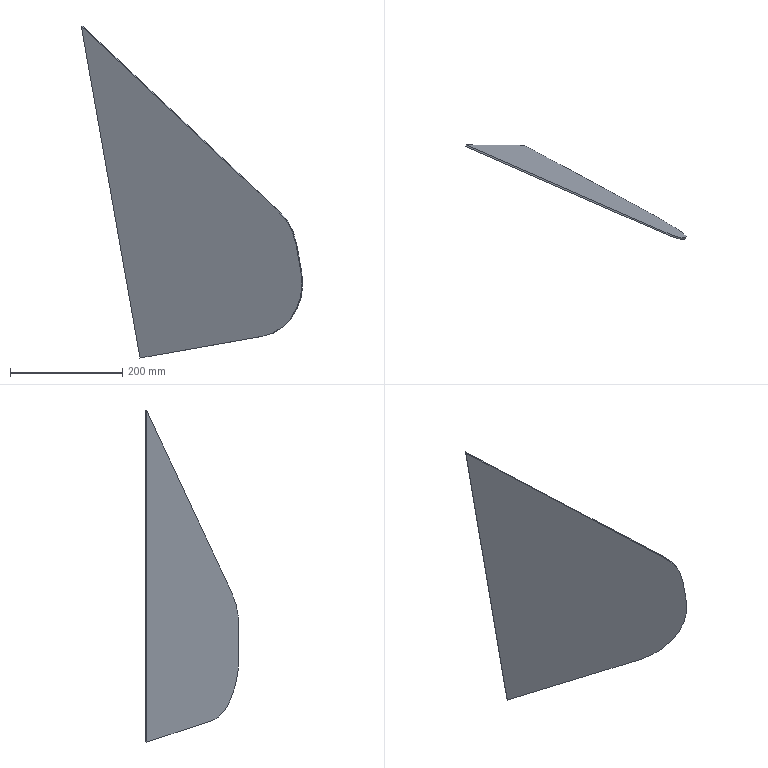Part | STEP file | floating channel right front section | 1 solid | 8 faces | box 394.503 x 166.964 x 591.584 mm | volume 406716 mm3 | plane 6 | cylinder 2 | commonest cylinder face diameters 200 x2
STEP:
#1=CARTESIAN_POINT('',(0.,0.,0.));
#2=DIRECTION('',(0.,0.,1.));
#3=DIRECTION('',(1.,0.,0.));
#4=AXIS2_PLACEMENT_3D('',#1,#2,#3);
#5=CARTESIAN_POINT('',(2381.907,-130.464,-318.268));
#6=VERTEX_POINT('',#5);
#7=CARTESIAN_POINT('',(2350.057,-119.338,-258.257));
#8=VERTEX_POINT('',#7);
#9=CARTESIAN_POINT('',(2294.958,-83.517,-333.629));
#10=DIRECTION('',(-0.4623,-0.8829,-0.08168));
#11=DIRECTION('',(0.8859,-0.4639,0.));
#12=AXIS2_PLACEMENT_3D('',#9,#10,#11);
#13=CIRCLE('',#12,100.);
#14=CARTESIAN_POINT('',(2294.958,-83.517,-333.629));
#15=DIRECTION('',(0.4623,0.8829,0.08168));
#16=DIRECTION('',(0.8859,-0.4639,0.));
#17=AXIS2_PLACEMENT_3D('',#14,#15,#16);
#18=CYLINDRICAL_SURFACE('',#17,100.);
#19=CARTESIAN_POINT('',(6.283,0.));
#20=DIRECTION('',(-1.,0.));
#21=VECTOR('',#20,1.);
#22=LINE('',#19,#21);
#23=(GEOMETRIC_REPRESENTATION_CONTEXT(2)PARAMETRIC_REPRESENTATION_CONTEXT()REPRESENTATION_CONTEXT('',''));
#24=DEFINITIONAL_REPRESENTATION('',(#22),#23);
#25=PCURVE('',#18,#24);
#26=CARTESIAN_POINT('',(443.818,847.627,78.409));
#27=DIRECTION('',(-0.4623,-0.8829,-0.08168));
#28=DIRECTION('',(-0.8859,0.4639,0.));
#29=AXIS2_PLACEMENT_3D('',#26,#27,#28);
#30=PLANE('',#29);
#31=CARTESIAN_POINT('',(-2071.861,413.419));
#32=DIRECTION('',(-1.,0.));
#33=AXIS2_PLACEMENT_2D('',#31,#32);
#34=CIRCLE('',#33,100.);
#35=(GEOMETRIC_REPRESENTATION_CONTEXT(2)PARAMETRIC_REPRESENTATION_CONTEXT()REPRESENTATION_CONTEXT('',''));
#36=DEFINITIONAL_REPRESENTATION('',(#34),#35);
#37=PCURVE('',#30,#36);
#38=SURFACE_CURVE('',#13,(#25,#37),.PCURVE_S1.);
#39=EDGE_CURVE('',#6,#8,#38,.T.);
#40=ORIENTED_EDGE('',*,*,#39,.F.);
#41=CARTESIAN_POINT('',(2383.294,-127.815,-318.023));
#42=VERTEX_POINT('',#41);
#43=CARTESIAN_POINT('',(2381.907,-130.464,-318.268));
#44=DIRECTION('',(-0.4623,-0.8829,-0.08168));
#45=VECTOR('',#44,1.);
#46=LINE('',#43,#45);
#47=CARTESIAN_POINT('',(6.128,0.));
#48=DIRECTION('',(0.,-1.));
#49=VECTOR('',#48,1.);
#50=LINE('',#47,#49);
#51=(GEOMETRIC_REPRESENTATION_CONTEXT(2)PARAMETRIC_REPRESENTATION_CONTEXT()REPRESENTATION_CONTEXT('',''));
#52=DEFINITIONAL_REPRESENTATION('',(#50),#51);
#53=PCURVE('',#18,#52);
#54=CARTESIAN_POINT('',(2408.119,-130.464,-466.64));
#55=DIRECTION('',(-0.8695,0.4695,-0.1536));
#56=DIRECTION('',(0.4751,0.8799,0.));
#57=AXIS2_PLACEMENT_3D('',#54,#55,#56);
#58=PLANE('',#57);
#59=CARTESIAN_POINT('',(-12.454,-150.154));
#60=DIRECTION('',(-0.9966,0.08266));
#61=VECTOR('',#60,1.);
#62=LINE('',#59,#61);
#63=(GEOMETRIC_REPRESENTATION_CONTEXT(2)PARAMETRIC_REPRESENTATION_CONTEXT()REPRESENTATION_CONTEXT('',''));
#64=DEFINITIONAL_REPRESENTATION('',(#62),#63);
#65=PCURVE('',#58,#64);
#66=SURFACE_CURVE('',#46,(#53,#65),.PCURVE_S1.);
#67=EDGE_CURVE('',#42,#6,#66,.T.);
#68=ORIENTED_EDGE('',*,*,#67,.F.);
#69=CARTESIAN_POINT('',(2351.444,-116.69,-258.012));
#70=VERTEX_POINT('',#69);
#71=CARTESIAN_POINT('',(2296.345,-80.868,-333.384));
#72=DIRECTION('',(0.4623,0.8829,0.08168));
#73=DIRECTION('',(0.8859,-0.4639,0.));
#74=AXIS2_PLACEMENT_3D('',#71,#72,#73);
#75=CIRCLE('',#74,100.);
#76=CARTESIAN_POINT('',(0.,3.));
#77=DIRECTION('',(1.,0.));
#78=VECTOR('',#77,1.);
#79=LINE('',#76,#78);
#80=(GEOMETRIC_REPRESENTATION_CONTEXT(2)PARAMETRIC_REPRESENTATION_CONTEXT()REPRESENTATION_CONTEXT('',''));
#81=DEFINITIONAL_REPRESENTATION('',(#79),#80);
#82=PCURVE('',#18,#81);
#83=CARTESIAN_POINT('',(445.205,850.276,78.654));
#84=DIRECTION('',(-0.4623,-0.8829,-0.08168));
#85=DIRECTION('',(-0.8859,0.4639,0.));
#86=AXIS2_PLACEMENT_3D('',#83,#84,#85);
#87=PLANE('',#86);
#88=CARTESIAN_POINT('',(-2171.861,413.419));
#89=CARTESIAN_POINT('',(-2171.861,586.624));
#90=CARTESIAN_POINT('',(-2021.861,500.022));
#91=CARTESIAN_POINT('',(-1871.861,413.419));
#92=CARTESIAN_POINT('',(-2021.861,326.816));
#93=CARTESIAN_POINT('',(-2171.861,240.214));
#94=CARTESIAN_POINT('',(-2171.861,413.419));
#95=(BOUNDED_CURVE()B_SPLINE_CURVE(2,(#88,#89,#90,#91,#92,#93,#94),.UNSPECIFIED.,.T.,.F.)B_SPLINE_CURVE_WITH_KNOTS((1,2,2,2,2,1),(-2.094,0.,2.094,4.189,6.283,8.378),.UNSPECIFIED.)CURVE()GEOMETRIC_REPRESENTATION_ITEM()RATIONAL_B_SPLINE_CURVE((1.,0.5,1.,0.5,1.,0.5,1.))REPRESENTATION_ITEM(''));
#96=(GEOMETRIC_REPRESENTATION_CONTEXT(2)PARAMETRIC_REPRESENTATION_CONTEXT()REPRESENTATION_CONTEXT('',''));
#97=DEFINITIONAL_REPRESENTATION('',(#95),#96);
#98=PCURVE('',#87,#97);
#99=SURFACE_CURVE('',#75,(#82,#98),.PCURVE_S1.);
#100=EDGE_CURVE('',#70,#42,#99,.T.);
#101=ORIENTED_EDGE('',*,*,#100,.F.);
#102=CARTESIAN_POINT('',(2350.057,-119.338,-258.257));
#103=DIRECTION('',(0.4623,0.8829,0.08168));
#104=VECTOR('',#103,1.);
#105=LINE('',#102,#104);
#106=CARTESIAN_POINT('',(5.426,0.));
#107=DIRECTION('',(0.,1.));
#108=VECTOR('',#107,1.);
#109=LINE('',#106,#108);
#110=(GEOMETRIC_REPRESENTATION_CONTEXT(2)PARAMETRIC_REPRESENTATION_CONTEXT()REPRESENTATION_CONTEXT('',''));
#111=DEFINITIONAL_REPRESENTATION('',(#109),#110);
#112=PCURVE('',#18,#111);
#113=CARTESIAN_POINT('',(2375.528,-130.464,-282.164));
#114=DIRECTION('',(-0.551,0.3582,-0.7537));
#115=DIRECTION('',(0.8073,0.,-0.5901));
#116=AXIS2_PLACEMENT_3D('',#113,#114,#115);
#117=PLANE('',#116);
#118=CARTESIAN_POINT('',(-34.672,-11.916));
#119=DIRECTION('',(0.325,-0.9457));
#120=VECTOR('',#119,1.);
#121=LINE('',#118,#120);
#122=(GEOMETRIC_REPRESENTATION_CONTEXT(2)PARAMETRIC_REPRESENTATION_CONTEXT()REPRESENTATION_CONTEXT('',''));
#123=DEFINITIONAL_REPRESENTATION('',(#121),#122);
#124=PCURVE('',#117,#123);
#125=SURFACE_CURVE('',#105,(#112,#124),.PCURVE_S1.);
#126=EDGE_CURVE('',#8,#70,#125,.T.);
#127=ORIENTED_EDGE('',*,*,#126,.F.);
#128=EDGE_LOOP('',(#40,#68,#101,#127));
#129=FACE_BOUND('',#128,.T.);
#130=ADVANCED_FACE('',(#129),#18,.T.);
#131=CARTESIAN_POINT('',(2321.171,-83.517,-482.001));
#132=VERTEX_POINT('',#131);
#133=CARTESIAN_POINT('',(2390.722,-130.464,-368.165));
#134=VERTEX_POINT('',#133);
#135=CARTESIAN_POINT('',(2303.774,-83.517,-383.526));
#136=DIRECTION('',(-0.4623,-0.8829,-0.08168));
#137=DIRECTION('',(0.8859,-0.4639,0.));
#138=AXIS2_PLACEMENT_3D('',#135,#136,#137);
#139=CIRCLE('',#138,100.);
#140=CARTESIAN_POINT('',(2303.774,-83.517,-383.526));
#141=DIRECTION('',(0.4623,0.8829,0.08168));
#142=DIRECTION('',(0.8859,-0.4639,0.));
#143=AXIS2_PLACEMENT_3D('',#140,#141,#142);
#144=CYLINDRICAL_SURFACE('',#143,100.);
#145=CARTESIAN_POINT('',(6.283,0.));
#146=DIRECTION('',(-1.,0.));
#147=VECTOR('',#146,1.);
#148=LINE('',#145,#147);
#149=(GEOMETRIC_REPRESENTATION_CONTEXT(2)PARAMETRIC_REPRESENTATION_CONTEXT()REPRESENTATION_CONTEXT('',''));
#150=DEFINITIONAL_REPRESENTATION('',(#148),#149);
#151=PCURVE('',#144,#150);
#152=CARTESIAN_POINT('',(-2079.671,463.483));
#153=DIRECTION('',(-1.,0.));
#154=AXIS2_PLACEMENT_2D('',#152,#153);
#155=CIRCLE('',#154,100.);
#156=(GEOMETRIC_REPRESENTATION_CONTEXT(2)PARAMETRIC_REPRESENTATION_CONTEXT()REPRESENTATION_CONTEXT('',''));
#157=DEFINITIONAL_REPRESENTATION('',(#155),#156);
#158=PCURVE('',#30,#157);
#159=SURFACE_CURVE('',#139,(#151,#158),.PCURVE_S1.);
#160=EDGE_CURVE('',#132,#134,#159,.T.);
#161=ORIENTED_EDGE('',*,*,#160,.F.);
#162=CARTESIAN_POINT('',(2322.558,-80.868,-481.756));
#163=VERTEX_POINT('',#162);
#164=CARTESIAN_POINT('',(2321.171,-83.517,-482.001));
#165=DIRECTION('',(-0.4623,-0.8829,-0.08168));
#166=VECTOR('',#165,1.);
#167=LINE('',#164,#166);
#168=CARTESIAN_POINT('',(1.416,0.));
#169=DIRECTION('',(0.,-1.));
#170=VECTOR('',#169,1.);
#171=LINE('',#168,#170);
#172=(GEOMETRIC_REPRESENTATION_CONTEXT(2)PARAMETRIC_REPRESENTATION_CONTEXT()REPRESENTATION_CONTEXT('',''));
#173=DEFINITIONAL_REPRESENTATION('',(#171),#172);
#174=PCURVE('',#144,#173);
#175=CARTESIAN_POINT('',(2103.8,33.851,-520.404));
#176=DIRECTION('',(-0.174,0.,0.9848));
#177=DIRECTION('',(-0.9848,0.,-0.174));
#178=AXIS2_PLACEMENT_3D('',#175,#176,#177);
#179=PLANE('',#178);
#180=CARTESIAN_POINT('',(-220.737,117.368));
#181=DIRECTION('',(0.4695,0.8829));
#182=VECTOR('',#181,1.);
#183=LINE('',#180,#182);
#184=(GEOMETRIC_REPRESENTATION_CONTEXT(2)PARAMETRIC_REPRESENTATION_CONTEXT()REPRESENTATION_CONTEXT('',''));
#185=DEFINITIONAL_REPRESENTATION('',(#183),#184);
#186=PCURVE('',#179,#185);
#187=SURFACE_CURVE('',#167,(#174,#186),.PCURVE_S1.);
#188=EDGE_CURVE('',#163,#132,#187,.T.);
#189=ORIENTED_EDGE('',*,*,#188,.F.);
#190=CARTESIAN_POINT('',(2392.109,-127.815,-367.92));
#191=VERTEX_POINT('',#190);
#192=CARTESIAN_POINT('',(2305.161,-80.868,-383.281));
#193=DIRECTION('',(0.4623,0.8829,0.08168));
#194=DIRECTION('',(0.8859,-0.4639,0.));
#195=AXIS2_PLACEMENT_3D('',#192,#193,#194);
#196=CIRCLE('',#195,100.);
#197=CARTESIAN_POINT('',(-6.283,3.));
#198=DIRECTION('',(1.,0.));
#199=VECTOR('',#198,1.);
#200=LINE('',#197,#199);
#201=(GEOMETRIC_REPRESENTATION_CONTEXT(2)PARAMETRIC_REPRESENTATION_CONTEXT()REPRESENTATION_CONTEXT('',''));
#202=DEFINITIONAL_REPRESENTATION('',(#200),#201);
#203=PCURVE('',#144,#202);
#204=CARTESIAN_POINT('',(-2179.671,463.483));
#205=CARTESIAN_POINT('',(-2179.671,636.688));
#206=CARTESIAN_POINT('',(-2029.671,550.086));
#207=CARTESIAN_POINT('',(-1879.671,463.483));
#208=CARTESIAN_POINT('',(-2029.671,376.881));
#209=CARTESIAN_POINT('',(-2179.671,290.278));
#210=CARTESIAN_POINT('',(-2179.671,463.483));
#211=(BOUNDED_CURVE()B_SPLINE_CURVE(2,(#204,#205,#206,#207,#208,#209,#210),.UNSPECIFIED.,.T.,.F.)B_SPLINE_CURVE_WITH_KNOTS((1,2,2,2,2,1),(-2.094,0.,2.094,4.189,6.283,8.378),.UNSPECIFIED.)CURVE()GEOMETRIC_REPRESENTATION_ITEM()RATIONAL_B_SPLINE_CURVE((1.,0.5,1.,0.5,1.,0.5,1.))REPRESENTATION_ITEM(''));
#212=(GEOMETRIC_REPRESENTATION_CONTEXT(2)PARAMETRIC_REPRESENTATION_CONTEXT()REPRESENTATION_CONTEXT('',''));
#213=DEFINITIONAL_REPRESENTATION('',(#211),#212);
#214=PCURVE('',#87,#213);
#215=SURFACE_CURVE('',#196,(#203,#214),.PCURVE_S1.);
#216=EDGE_CURVE('',#191,#163,#215,.T.);
#217=ORIENTED_EDGE('',*,*,#216,.F.);
#218=CARTESIAN_POINT('',(2390.722,-130.464,-368.165));
#219=DIRECTION('',(0.4623,0.8829,0.08168));
#220=VECTOR('',#219,1.);
#221=LINE('',#218,#220);
#222=CARTESIAN_POINT('',(-0.1547,0.));
#223=DIRECTION('',(0.,1.));
#224=VECTOR('',#223,1.);
#225=LINE('',#222,#224);
#226=(GEOMETRIC_REPRESENTATION_CONTEXT(2)PARAMETRIC_REPRESENTATION_CONTEXT()REPRESENTATION_CONTEXT('',''));
#227=DEFINITIONAL_REPRESENTATION('',(#225),#226);
#228=PCURVE('',#144,#227);
#229=CARTESIAN_POINT('',(-8.266,-99.658));
#230=DIRECTION('',(0.9966,-0.08266));
#231=VECTOR('',#230,1.);
#232=LINE('',#229,#231);
#233=(GEOMETRIC_REPRESENTATION_CONTEXT(2)PARAMETRIC_REPRESENTATION_CONTEXT()REPRESENTATION_CONTEXT('',''));
#234=DEFINITIONAL_REPRESENTATION('',(#232),#233);
#235=PCURVE('',#58,#234);
#236=SURFACE_CURVE('',#221,(#228,#235),.PCURVE_S1.);
#237=EDGE_CURVE('',#134,#191,#236,.T.);
#238=ORIENTED_EDGE('',*,*,#237,.F.);
#239=EDGE_LOOP('',(#161,#189,#217,#238));
#240=FACE_BOUND('',#239,.T.);
#241=ADVANCED_FACE('',(#240),#144,.T.);
#242=CARTESIAN_POINT('',(2000.716,36.5,71.181));
#243=VERTEX_POINT('',#242);
#244=CARTESIAN_POINT('',(2376.915,-127.815,-281.919));
#245=DIRECTION('',(-0.6948,0.3035,0.6521));
#246=VECTOR('',#245,1.);
#247=LINE('',#244,#246);
#248=CARTESIAN_POINT('',(-2165.016,361.782));
#249=DIRECTION('',(0.7562,-0.6543));
#250=VECTOR('',#249,1.);
#251=LINE('',#248,#250);
#252=(GEOMETRIC_REPRESENTATION_CONTEXT(2)PARAMETRIC_REPRESENTATION_CONTEXT()REPRESENTATION_CONTEXT('',''));
#253=DEFINITIONAL_REPRESENTATION('',(#251),#252);
#254=PCURVE('',#87,#253);
#255=CARTESIAN_POINT('',(0.9751,-2.837));
#256=DIRECTION('',(-0.9457,-0.325));
#257=VECTOR('',#256,1.);
#258=LINE('',#255,#257);
#259=(GEOMETRIC_REPRESENTATION_CONTEXT(2)PARAMETRIC_REPRESENTATION_CONTEXT()REPRESENTATION_CONTEXT('',''));
#260=DEFINITIONAL_REPRESENTATION('',(#258),#259);
#261=PCURVE('',#117,#260);
#262=SURFACE_CURVE('',#247,(#254,#261),.PCURVE_S1.);
#263=EDGE_CURVE('',#70,#243,#262,.T.);
#264=ORIENTED_EDGE('',*,*,#263,.F.);
#265=ORIENTED_EDGE('',*,*,#100,.T.);
#266=CARTESIAN_POINT('',(2409.506,-127.815,-466.395));
#267=DIRECTION('',(-0.174,0.,0.9848));
#268=VECTOR('',#267,1.);
#269=LINE('',#266,#268);
#270=CARTESIAN_POINT('',(-2193.888,546.876));
#271=DIRECTION('',(0.1541,-0.9881));
#272=VECTOR('',#271,1.);
#273=LINE('',#270,#272);
#274=(GEOMETRIC_REPRESENTATION_CONTEXT(2)PARAMETRIC_REPRESENTATION_CONTEXT()REPRESENTATION_CONTEXT('',''));
#275=DEFINITIONAL_REPRESENTATION('',(#273),#274);
#276=PCURVE('',#87,#275);
#277=CARTESIAN_POINT('',(2.99,-0.248));
#278=DIRECTION('',(-0.08266,-0.9966));
#279=VECTOR('',#278,1.);
#280=LINE('',#277,#279);
#281=(GEOMETRIC_REPRESENTATION_CONTEXT(2)PARAMETRIC_REPRESENTATION_CONTEXT()REPRESENTATION_CONTEXT('',''));
#282=DEFINITIONAL_REPRESENTATION('',(#280),#281);
#283=PCURVE('',#58,#282);
#284=SURFACE_CURVE('',#269,(#276,#283),.PCURVE_S1.);
#285=EDGE_CURVE('',#191,#42,#284,.T.);
#286=ORIENTED_EDGE('',*,*,#285,.F.);
#287=ORIENTED_EDGE('',*,*,#216,.T.);
#288=CARTESIAN_POINT('',(2105.187,36.5,-520.159));
#289=VERTEX_POINT('',#288);
#290=CARTESIAN_POINT('',(2105.187,36.5,-520.159));
#291=DIRECTION('',(0.8695,-0.4695,0.1536));
#292=VECTOR('',#291,1.);
#293=LINE('',#290,#292);
#294=CARTESIAN_POINT('',(-1848.07,600.82));
#295=DIRECTION('',(-0.9881,-0.1541));
#296=VECTOR('',#295,1.);
#297=LINE('',#294,#296);
#298=(GEOMETRIC_REPRESENTATION_CONTEXT(2)PARAMETRIC_REPRESENTATION_CONTEXT()REPRESENTATION_CONTEXT('',''));
#299=DEFINITIONAL_REPRESENTATION('',(#297),#298);
#300=PCURVE('',#87,#299);
#301=CARTESIAN_POINT('',(-1.408,-2.649));
#302=DIRECTION('',(-0.8829,0.4695));
#303=VECTOR('',#302,1.);
#304=LINE('',#301,#303);
#305=(GEOMETRIC_REPRESENTATION_CONTEXT(2)PARAMETRIC_REPRESENTATION_CONTEXT()REPRESENTATION_CONTEXT('',''));
#306=DEFINITIONAL_REPRESENTATION('',(#304),#305);
#307=PCURVE('',#179,#306);
#308=SURFACE_CURVE('',#293,(#300,#307),.PCURVE_S1.);
#309=EDGE_CURVE('',#289,#163,#308,.T.);
#310=ORIENTED_EDGE('',*,*,#309,.F.);
#311=CARTESIAN_POINT('',(2000.716,36.5,71.181));
#312=DIRECTION('',(0.174,0.,-0.9848));
#313=VECTOR('',#312,1.);
#314=LINE('',#311,#313);
#315=CARTESIAN_POINT('',(-1755.518,7.498));
#316=DIRECTION('',(-0.1541,0.9881));
#317=VECTOR('',#316,1.);
#318=LINE('',#315,#317);
#319=(GEOMETRIC_REPRESENTATION_CONTEXT(2)PARAMETRIC_REPRESENTATION_CONTEXT()REPRESENTATION_CONTEXT('',''));
#320=DEFINITIONAL_REPRESENTATION('',(#318),#319);
#321=PCURVE('',#87,#320);
#322=CARTESIAN_POINT('',(1999.329,33.851,70.936));
#323=DIRECTION('',(0.8695,-0.4695,0.1536));
#324=DIRECTION('',(-0.4751,-0.8799,0.));
#325=AXIS2_PLACEMENT_3D('',#322,#323,#324);
#326=PLANE('',#325);
#327=CARTESIAN_POINT('',(-2.99,-0.248));
#328=DIRECTION('',(-0.08266,0.9966));
#329=VECTOR('',#328,1.);
#330=LINE('',#327,#329);
#331=(GEOMETRIC_REPRESENTATION_CONTEXT(2)PARAMETRIC_REPRESENTATION_CONTEXT()REPRESENTATION_CONTEXT('',''));
#332=DEFINITIONAL_REPRESENTATION('',(#330),#331);
#333=PCURVE('',#326,#332);
#334=SURFACE_CURVE('',#314,(#321,#333),.PCURVE_S1.);
#335=EDGE_CURVE('',#243,#289,#334,.T.);
#336=ORIENTED_EDGE('',*,*,#335,.F.);
#337=EDGE_LOOP('',(#264,#265,#286,#287,#310,#336));
#338=FACE_BOUND('',#337,.T.);
#339=ADVANCED_FACE('',(#338),#87,.F.);
#340=CARTESIAN_POINT('',(2408.119,-130.464,-466.64));
#341=DIRECTION('',(-0.174,0.,0.9848));
#342=VECTOR('',#341,1.);
#343=LINE('',#340,#342);
#344=CARTESIAN_POINT('',(-2193.888,546.876));
#345=DIRECTION('',(0.1541,-0.9881));
#346=VECTOR('',#345,1.);
#347=LINE('',#344,#346);
#348=(GEOMETRIC_REPRESENTATION_CONTEXT(2)PARAMETRIC_REPRESENTATION_CONTEXT()REPRESENTATION_CONTEXT('',''));
#349=DEFINITIONAL_REPRESENTATION('',(#347),#348);
#350=PCURVE('',#30,#349);
#351=CARTESIAN_POINT('',(0.,0.));
#352=DIRECTION('',(-0.08266,-0.9966));
#353=VECTOR('',#352,1.);
#354=LINE('',#351,#353);
#355=(GEOMETRIC_REPRESENTATION_CONTEXT(2)PARAMETRIC_REPRESENTATION_CONTEXT()REPRESENTATION_CONTEXT('',''));
#356=DEFINITIONAL_REPRESENTATION('',(#354),#355);
#357=PCURVE('',#58,#356);
#358=SURFACE_CURVE('',#343,(#350,#357),.PCURVE_S1.);
#359=EDGE_CURVE('',#134,#6,#358,.T.);
#360=ORIENTED_EDGE('',*,*,#359,.T.);
#361=ORIENTED_EDGE('',*,*,#39,.T.);
#362=CARTESIAN_POINT('',(1999.329,33.851,70.936));
#363=VERTEX_POINT('',#362);
#364=CARTESIAN_POINT('',(2375.528,-130.464,-282.164));
#365=DIRECTION('',(-0.6948,0.3035,0.6521));
#366=VECTOR('',#365,1.);
#367=LINE('',#364,#366);
#368=CARTESIAN_POINT('',(-2165.016,361.782));
#369=DIRECTION('',(0.7562,-0.6543));
#370=VECTOR('',#369,1.);
#371=LINE('',#368,#370);
#372=(GEOMETRIC_REPRESENTATION_CONTEXT(2)PARAMETRIC_REPRESENTATION_CONTEXT()REPRESENTATION_CONTEXT('',''));
#373=DEFINITIONAL_REPRESENTATION('',(#371),#372);
#374=PCURVE('',#30,#373);
#375=CARTESIAN_POINT('',(0.,0.));
#376=DIRECTION('',(-0.9457,-0.325));
#377=VECTOR('',#376,1.);
#378=LINE('',#375,#377);
#379=(GEOMETRIC_REPRESENTATION_CONTEXT(2)PARAMETRIC_REPRESENTATION_CONTEXT()REPRESENTATION_CONTEXT('',''));
#380=DEFINITIONAL_REPRESENTATION('',(#378),#379);
#381=PCURVE('',#117,#380);
#382=SURFACE_CURVE('',#367,(#374,#381),.PCURVE_S1.);
#383=EDGE_CURVE('',#8,#363,#382,.T.);
#384=ORIENTED_EDGE('',*,*,#383,.T.);
#385=CARTESIAN_POINT('',(2103.8,33.851,-520.404));
#386=VERTEX_POINT('',#385);
#387=CARTESIAN_POINT('',(1999.329,33.851,70.936));
#388=DIRECTION('',(0.174,0.,-0.9848));
#389=VECTOR('',#388,1.);
#390=LINE('',#387,#389);
#391=CARTESIAN_POINT('',(-1755.518,7.498));
#392=DIRECTION('',(-0.1541,0.9881));
#393=VECTOR('',#392,1.);
#394=LINE('',#391,#393);
#395=(GEOMETRIC_REPRESENTATION_CONTEXT(2)PARAMETRIC_REPRESENTATION_CONTEXT()REPRESENTATION_CONTEXT('',''));
#396=DEFINITIONAL_REPRESENTATION('',(#394),#395);
#397=PCURVE('',#30,#396);
#398=CARTESIAN_POINT('',(0.,0.));
#399=DIRECTION('',(-0.08266,0.9966));
#400=VECTOR('',#399,1.);
#401=LINE('',#398,#400);
#402=(GEOMETRIC_REPRESENTATION_CONTEXT(2)PARAMETRIC_REPRESENTATION_CONTEXT()REPRESENTATION_CONTEXT('',''));
#403=DEFINITIONAL_REPRESENTATION('',(#401),#402);
#404=PCURVE('',#326,#403);
#405=SURFACE_CURVE('',#390,(#397,#404),.PCURVE_S1.);
#406=EDGE_CURVE('',#363,#386,#405,.T.);
#407=ORIENTED_EDGE('',*,*,#406,.T.);
#408=CARTESIAN_POINT('',(2103.8,33.851,-520.404));
#409=DIRECTION('',(0.8695,-0.4695,0.1536));
#410=VECTOR('',#409,1.);
#411=LINE('',#408,#410);
#412=CARTESIAN_POINT('',(-1848.07,600.82));
#413=DIRECTION('',(-0.9881,-0.1541));
#414=VECTOR('',#413,1.);
#415=LINE('',#412,#414);
#416=(GEOMETRIC_REPRESENTATION_CONTEXT(2)PARAMETRIC_REPRESENTATION_CONTEXT()REPRESENTATION_CONTEXT('',''));
#417=DEFINITIONAL_REPRESENTATION('',(#415),#416);
#418=PCURVE('',#30,#417);
#419=CARTESIAN_POINT('',(0.,0.));
#420=DIRECTION('',(-0.8829,0.4695));
#421=VECTOR('',#420,1.);
#422=LINE('',#419,#421);
#423=(GEOMETRIC_REPRESENTATION_CONTEXT(2)PARAMETRIC_REPRESENTATION_CONTEXT()REPRESENTATION_CONTEXT('',''));
#424=DEFINITIONAL_REPRESENTATION('',(#422),#423);
#425=PCURVE('',#179,#424);
#426=SURFACE_CURVE('',#411,(#418,#425),.PCURVE_S1.);
#427=EDGE_CURVE('',#386,#132,#426,.T.);
#428=ORIENTED_EDGE('',*,*,#427,.T.);
#429=ORIENTED_EDGE('',*,*,#160,.T.);
#430=EDGE_LOOP('',(#360,#361,#384,#407,#428,#429));
#431=FACE_BOUND('',#430,.T.);
#432=ADVANCED_FACE('',(#431),#30,.T.);
#433=ORIENTED_EDGE('',*,*,#383,.F.);
#434=ORIENTED_EDGE('',*,*,#126,.T.);
#435=ORIENTED_EDGE('',*,*,#263,.T.);
#436=CARTESIAN_POINT('',(1999.329,33.851,70.936));
#437=DIRECTION('',(0.4623,0.8829,0.08168));
#438=VECTOR('',#437,1.);
#439=LINE('',#436,#438);
#440=CARTESIAN_POINT('',(-512.085,-175.994));
#441=DIRECTION('',(0.325,-0.9457));
#442=VECTOR('',#441,1.);
#443=LINE('',#440,#442);
#444=(GEOMETRIC_REPRESENTATION_CONTEXT(2)PARAMETRIC_REPRESENTATION_CONTEXT()REPRESENTATION_CONTEXT('',''));
#445=DEFINITIONAL_REPRESENTATION('',(#443),#444);
#446=PCURVE('',#117,#445);
#447=CARTESIAN_POINT('',(0.,0.));
#448=DIRECTION('',(-0.9966,-0.08266));
#449=VECTOR('',#448,1.);
#450=LINE('',#447,#449);
#451=(GEOMETRIC_REPRESENTATION_CONTEXT(2)PARAMETRIC_REPRESENTATION_CONTEXT()REPRESENTATION_CONTEXT('',''));
#452=DEFINITIONAL_REPRESENTATION('',(#450),#451);
#453=PCURVE('',#326,#452);
#454=SURFACE_CURVE('',#439,(#446,#453),.PCURVE_S1.);
#455=EDGE_CURVE('',#363,#243,#454,.T.);
#456=ORIENTED_EDGE('',*,*,#455,.F.);
#457=EDGE_LOOP('',(#433,#434,#435,#456));
#458=FACE_BOUND('',#457,.T.);
#459=ADVANCED_FACE('',(#458),#117,.F.);
#460=ORIENTED_EDGE('',*,*,#285,.T.);
#461=ORIENTED_EDGE('',*,*,#67,.T.);
#462=ORIENTED_EDGE('',*,*,#359,.F.);
#463=ORIENTED_EDGE('',*,*,#237,.T.);
#464=EDGE_LOOP('',(#460,#461,#462,#463));
#465=FACE_BOUND('',#464,.T.);
#466=ADVANCED_FACE('',(#465),#58,.F.);
#467=ORIENTED_EDGE('',*,*,#309,.T.);
#468=ORIENTED_EDGE('',*,*,#188,.T.);
#469=ORIENTED_EDGE('',*,*,#427,.F.);
#470=CARTESIAN_POINT('',(2103.8,33.851,-520.404));
#471=DIRECTION('',(0.4623,0.8829,0.08168));
#472=VECTOR('',#471,1.);
#473=LINE('',#470,#472);
#474=CARTESIAN_POINT('',(0.,0.));
#475=DIRECTION('',(-0.4695,-0.8829));
#476=VECTOR('',#475,1.);
#477=LINE('',#474,#476);
#478=(GEOMETRIC_REPRESENTATION_CONTEXT(2)PARAMETRIC_REPRESENTATION_CONTEXT()REPRESENTATION_CONTEXT('',''));
#479=DEFINITIONAL_REPRESENTATION('',(#477),#478);
#480=PCURVE('',#179,#479);
#481=CARTESIAN_POINT('',(-49.635,598.442));
#482=DIRECTION('',(-0.9966,-0.08266));
#483=VECTOR('',#482,1.);
#484=LINE('',#481,#483);
#485=(GEOMETRIC_REPRESENTATION_CONTEXT(2)PARAMETRIC_REPRESENTATION_CONTEXT()REPRESENTATION_CONTEXT('',''));
#486=DEFINITIONAL_REPRESENTATION('',(#484),#485);
#487=PCURVE('',#326,#486);
#488=SURFACE_CURVE('',#473,(#480,#487),.PCURVE_S1.);
#489=EDGE_CURVE('',#386,#289,#488,.T.);
#490=ORIENTED_EDGE('',*,*,#489,.T.);
#491=EDGE_LOOP('',(#467,#468,#469,#490));
#492=FACE_BOUND('',#491,.T.);
#493=ADVANCED_FACE('',(#492),#179,.F.);
#494=ORIENTED_EDGE('',*,*,#335,.T.);
#495=ORIENTED_EDGE('',*,*,#489,.F.);
#496=ORIENTED_EDGE('',*,*,#406,.F.);
#497=ORIENTED_EDGE('',*,*,#455,.T.);
#498=EDGE_LOOP('',(#494,#495,#496,#497));
#499=FACE_BOUND('',#498,.T.);
#500=ADVANCED_FACE('',(#499),#326,.F.);
#501=CLOSED_SHELL('',(#130,#241,#339,#432,#459,#466,#493,#500));
#502=MANIFOLD_SOLID_BREP('',#501);
#503=(LENGTH_UNIT()NAMED_UNIT(*)SI_UNIT(.MILLI.,.METRE.));
#504=UNCERTAINTY_MEASURE_WITH_UNIT(LENGTH_MEASURE(0.0000001),#503,'','');
#505=(NAMED_UNIT(*)PLANE_ANGLE_UNIT()SI_UNIT($,.RADIAN.));
#506=(NAMED_UNIT(*)SI_UNIT($,.STERADIAN.)SOLID_ANGLE_UNIT());
#507=(GEOMETRIC_REPRESENTATION_CONTEXT(3)GLOBAL_UNCERTAINTY_ASSIGNED_CONTEXT((#504))GLOBAL_UNIT_ASSIGNED_CONTEXT((#503,#505,#506))REPRESENTATION_CONTEXT('',''));
#508=ADVANCED_BREP_SHAPE_REPRESENTATION('',(#4,#502),#507);